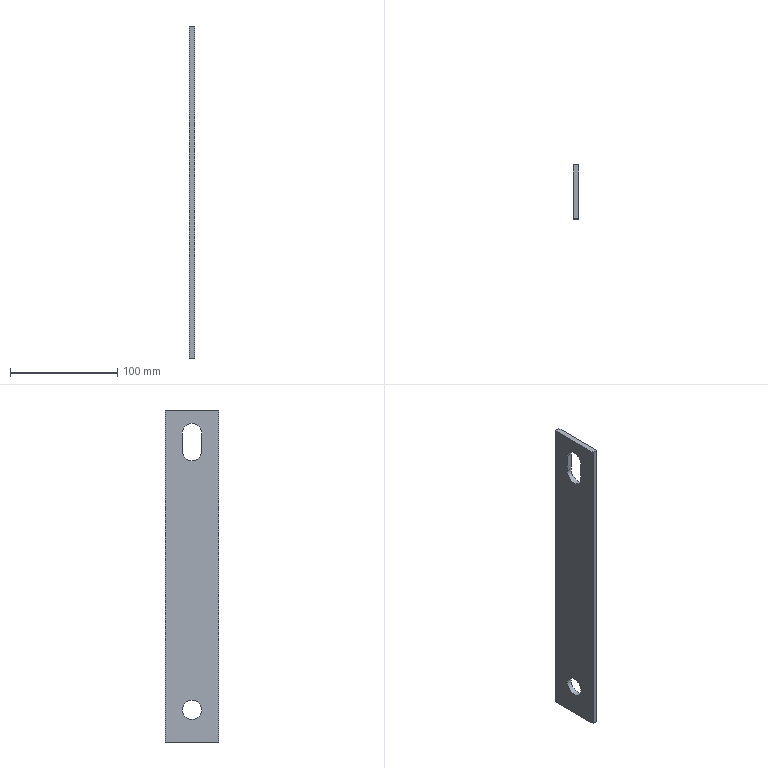Part | NX | features solid 2 | 1 solid | 11 faces | box 5 x 50 x 310 mm | volume 73425 mm3 | plane 8 | cylinder 3 | commonest cylinder face diameters 18 x3
STEP:
#1=CARTESIAN_POINT('',(-1060.,-545.,-129.));
#2=VERTEX_POINT('',#1);
#3=CARTESIAN_POINT('',(-1060.,-545.,181.));
#4=VERTEX_POINT('',#3);
#5=CARTESIAN_POINT('',(-1060.,-545.,-129.));
#6=DIRECTION('',(0.,0.,1.));
#7=VECTOR('',#6,1000.);
#8=LINE('',#5,#7);
#9=EDGE_CURVE('',#2,#4,#8,.T.);
#10=ORIENTED_EDGE('',*,*,#9,.T.);
#11=CARTESIAN_POINT('',(-1065.,-545.,181.));
#12=VERTEX_POINT('',#11);
#13=CARTESIAN_POINT('',(-1065.,-545.,181.));
#14=DIRECTION('',(1.,0.,0.));
#15=VECTOR('',#14,1000.);
#16=LINE('',#13,#15);
#17=EDGE_CURVE('',#12,#4,#16,.T.);
#18=ORIENTED_EDGE('',*,*,#17,.F.);
#19=CARTESIAN_POINT('',(-1065.,-545.,-129.));
#20=VERTEX_POINT('',#19);
#21=CARTESIAN_POINT('',(-1065.,-545.,-129.));
#22=DIRECTION('',(0.,0.,1.));
#23=VECTOR('',#22,1000.);
#24=LINE('',#21,#23);
#25=EDGE_CURVE('',#20,#12,#24,.T.);
#26=ORIENTED_EDGE('',*,*,#25,.F.);
#27=CARTESIAN_POINT('',(-1065.,-545.,-129.));
#28=DIRECTION('',(1.,0.,0.));
#29=VECTOR('',#28,1000.);
#30=LINE('',#27,#29);
#31=EDGE_CURVE('',#20,#2,#30,.T.);
#32=ORIENTED_EDGE('',*,*,#31,.T.);
#33=EDGE_LOOP('',(#10,#18,#26,#32));
#34=FACE_BOUND('',#33,.T.);
#35=CARTESIAN_POINT('',(-1065.,-545.,-129.));
#36=DIRECTION('',(0.,-1.,0.));
#37=DIRECTION('',(0.,0.,1.));
#38=AXIS2_PLACEMENT_3D('',#35,#36,#37);
#39=PLANE('',#38);
#40=ADVANCED_FACE('',(#34),#39,.T.);
#41=CARTESIAN_POINT('',(-1060.,-495.,181.));
#42=VERTEX_POINT('',#41);
#43=CARTESIAN_POINT('',(-1060.,-545.,181.));
#44=DIRECTION('',(0.,1.,0.));
#45=VECTOR('',#44,1000.);
#46=LINE('',#43,#45);
#47=EDGE_CURVE('',#4,#42,#46,.T.);
#48=ORIENTED_EDGE('',*,*,#47,.T.);
#49=CARTESIAN_POINT('',(-1065.,-495.,181.));
#50=VERTEX_POINT('',#49);
#51=CARTESIAN_POINT('',(-1065.,-495.,181.));
#52=DIRECTION('',(1.,0.,0.));
#53=VECTOR('',#52,1000.);
#54=LINE('',#51,#53);
#55=EDGE_CURVE('',#50,#42,#54,.T.);
#56=ORIENTED_EDGE('',*,*,#55,.F.);
#57=CARTESIAN_POINT('',(-1065.,-545.,181.));
#58=DIRECTION('',(0.,1.,0.));
#59=VECTOR('',#58,1000.);
#60=LINE('',#57,#59);
#61=EDGE_CURVE('',#12,#50,#60,.T.);
#62=ORIENTED_EDGE('',*,*,#61,.F.);
#63=ORIENTED_EDGE('',*,*,#17,.T.);
#64=EDGE_LOOP('',(#48,#56,#62,#63));
#65=FACE_BOUND('',#64,.T.);
#66=CARTESIAN_POINT('',(-1065.,-545.,181.));
#67=DIRECTION('',(0.,0.,1.));
#68=DIRECTION('',(1.,0.,0.));
#69=AXIS2_PLACEMENT_3D('',#66,#67,#68);
#70=PLANE('',#69);
#71=ADVANCED_FACE('',(#65),#70,.T.);
#72=CARTESIAN_POINT('',(-1060.,-495.,-129.));
#73=VERTEX_POINT('',#72);
#74=CARTESIAN_POINT('',(-1060.,-495.,181.));
#75=DIRECTION('',(0.,0.,-1.));
#76=VECTOR('',#75,1000.);
#77=LINE('',#74,#76);
#78=EDGE_CURVE('',#42,#73,#77,.T.);
#79=ORIENTED_EDGE('',*,*,#78,.T.);
#80=CARTESIAN_POINT('',(-1065.,-495.,-129.));
#81=VERTEX_POINT('',#80);
#82=CARTESIAN_POINT('',(-1065.,-495.,-129.));
#83=DIRECTION('',(1.,0.,0.));
#84=VECTOR('',#83,1000.);
#85=LINE('',#82,#84);
#86=EDGE_CURVE('',#81,#73,#85,.T.);
#87=ORIENTED_EDGE('',*,*,#86,.F.);
#88=CARTESIAN_POINT('',(-1065.,-495.,181.));
#89=DIRECTION('',(0.,0.,-1.));
#90=VECTOR('',#89,1000.);
#91=LINE('',#88,#90);
#92=EDGE_CURVE('',#50,#81,#91,.T.);
#93=ORIENTED_EDGE('',*,*,#92,.F.);
#94=ORIENTED_EDGE('',*,*,#55,.T.);
#95=EDGE_LOOP('',(#79,#87,#93,#94));
#96=FACE_BOUND('',#95,.T.);
#97=CARTESIAN_POINT('',(-1065.,-495.,181.));
#98=DIRECTION('',(0.,1.,0.));
#99=DIRECTION('',(0.,0.,-1.));
#100=AXIS2_PLACEMENT_3D('',#97,#98,#99);
#101=PLANE('',#100);
#102=ADVANCED_FACE('',(#96),#101,.T.);
#103=CARTESIAN_POINT('',(-1060.,-511.,142.5));
#104=VERTEX_POINT('',#103);
#105=CARTESIAN_POINT('',(-1060.,-529.,142.5));
#106=VERTEX_POINT('',#105);
#107=CARTESIAN_POINT('',(-1060.,-520.,142.5));
#108=DIRECTION('',(-1.,0.,0.));
#109=DIRECTION('',(0.,-1.,0.));
#110=AXIS2_PLACEMENT_3D('',#107,#108,#109);
#111=CIRCLE('',#110,9.);
#112=EDGE_CURVE('',#104,#106,#111,.T.);
#113=ORIENTED_EDGE('',*,*,#112,.F.);
#114=CARTESIAN_POINT('',(-1065.,-511.,142.5));
#115=VERTEX_POINT('',#114);
#116=CARTESIAN_POINT('',(-1065.,-511.,142.5));
#117=DIRECTION('',(1.,0.,0.));
#118=VECTOR('',#117,1000.);
#119=LINE('',#116,#118);
#120=EDGE_CURVE('',#115,#104,#119,.T.);
#121=ORIENTED_EDGE('',*,*,#120,.F.);
#122=CARTESIAN_POINT('',(-1065.,-529.,142.5));
#123=VERTEX_POINT('',#122);
#124=CARTESIAN_POINT('',(-1065.,-520.,142.5));
#125=DIRECTION('',(-1.,0.,0.));
#126=DIRECTION('',(0.,-1.,0.));
#127=AXIS2_PLACEMENT_3D('',#124,#125,#126);
#128=CIRCLE('',#127,9.);
#129=EDGE_CURVE('',#115,#123,#128,.T.);
#130=ORIENTED_EDGE('',*,*,#129,.T.);
#131=CARTESIAN_POINT('',(-1065.,-529.,142.5));
#132=DIRECTION('',(1.,0.,0.));
#133=VECTOR('',#132,1000.);
#134=LINE('',#131,#133);
#135=EDGE_CURVE('',#123,#106,#134,.T.);
#136=ORIENTED_EDGE('',*,*,#135,.T.);
#137=EDGE_LOOP('',(#113,#121,#130,#136));
#138=FACE_BOUND('',#137,.T.);
#139=CARTESIAN_POINT('',(-1065.,-520.,142.5));
#140=DIRECTION('',(1.,0.,0.));
#141=DIRECTION('',(0.,-1.,0.));
#142=AXIS2_PLACEMENT_3D('',#139,#140,#141);
#143=CYLINDRICAL_SURFACE('',#142,9.);
#144=ADVANCED_FACE('',(#138),#143,.F.);
#145=CARTESIAN_POINT('',(-1060.,-511.,159.5));
#146=VERTEX_POINT('',#145);
#147=CARTESIAN_POINT('',(-1060.,-511.,142.5));
#148=DIRECTION('',(0.,0.,1.));
#149=VECTOR('',#148,1000.);
#150=LINE('',#147,#149);
#151=EDGE_CURVE('',#104,#146,#150,.T.);
#152=ORIENTED_EDGE('',*,*,#151,.T.);
#153=CARTESIAN_POINT('',(-1065.,-511.,159.5));
#154=VERTEX_POINT('',#153);
#155=CARTESIAN_POINT('',(-1065.,-511.,159.5));
#156=DIRECTION('',(1.,0.,0.));
#157=VECTOR('',#156,1000.);
#158=LINE('',#155,#157);
#159=EDGE_CURVE('',#154,#146,#158,.T.);
#160=ORIENTED_EDGE('',*,*,#159,.F.);
#161=CARTESIAN_POINT('',(-1065.,-511.,142.5));
#162=DIRECTION('',(0.,0.,1.));
#163=VECTOR('',#162,1000.);
#164=LINE('',#161,#163);
#165=EDGE_CURVE('',#115,#154,#164,.T.);
#166=ORIENTED_EDGE('',*,*,#165,.F.);
#167=ORIENTED_EDGE('',*,*,#120,.T.);
#168=EDGE_LOOP('',(#152,#160,#166,#167));
#169=FACE_BOUND('',#168,.T.);
#170=CARTESIAN_POINT('',(-1065.,-511.,142.5));
#171=DIRECTION('',(0.,-1.,0.));
#172=DIRECTION('',(-1.,0.,0.));
#173=AXIS2_PLACEMENT_3D('',#170,#171,#172);
#174=PLANE('',#173);
#175=ADVANCED_FACE('',(#169),#174,.T.);
#176=CARTESIAN_POINT('',(-1060.,-529.,159.5));
#177=VERTEX_POINT('',#176);
#178=CARTESIAN_POINT('',(-1060.,-520.,159.5));
#179=DIRECTION('',(-1.,0.,0.));
#180=DIRECTION('',(0.,-1.,0.));
#181=AXIS2_PLACEMENT_3D('',#178,#179,#180);
#182=CIRCLE('',#181,9.);
#183=EDGE_CURVE('',#177,#146,#182,.T.);
#184=ORIENTED_EDGE('',*,*,#183,.F.);
#185=CARTESIAN_POINT('',(-1065.,-529.,159.5));
#186=VERTEX_POINT('',#185);
#187=CARTESIAN_POINT('',(-1065.,-529.,159.5));
#188=DIRECTION('',(1.,0.,0.));
#189=VECTOR('',#188,1000.);
#190=LINE('',#187,#189);
#191=EDGE_CURVE('',#186,#177,#190,.T.);
#192=ORIENTED_EDGE('',*,*,#191,.F.);
#193=CARTESIAN_POINT('',(-1065.,-520.,159.5));
#194=DIRECTION('',(-1.,0.,0.));
#195=DIRECTION('',(0.,-1.,0.));
#196=AXIS2_PLACEMENT_3D('',#193,#194,#195);
#197=CIRCLE('',#196,9.);
#198=EDGE_CURVE('',#186,#154,#197,.T.);
#199=ORIENTED_EDGE('',*,*,#198,.T.);
#200=ORIENTED_EDGE('',*,*,#159,.T.);
#201=EDGE_LOOP('',(#184,#192,#199,#200));
#202=FACE_BOUND('',#201,.T.);
#203=CARTESIAN_POINT('',(-1065.,-520.,159.5));
#204=DIRECTION('',(1.,0.,0.));
#205=DIRECTION('',(0.,-1.,0.));
#206=AXIS2_PLACEMENT_3D('',#203,#204,#205);
#207=CYLINDRICAL_SURFACE('',#206,9.);
#208=ADVANCED_FACE('',(#202),#207,.F.);
#209=CARTESIAN_POINT('',(-1060.,-529.,159.5));
#210=DIRECTION('',(0.,0.,-1.));
#211=VECTOR('',#210,1000.);
#212=LINE('',#209,#211);
#213=EDGE_CURVE('',#177,#106,#212,.T.);
#214=ORIENTED_EDGE('',*,*,#213,.T.);
#215=ORIENTED_EDGE('',*,*,#135,.F.);
#216=CARTESIAN_POINT('',(-1065.,-529.,159.5));
#217=DIRECTION('',(0.,0.,-1.));
#218=VECTOR('',#217,1000.);
#219=LINE('',#216,#218);
#220=EDGE_CURVE('',#186,#123,#219,.T.);
#221=ORIENTED_EDGE('',*,*,#220,.F.);
#222=ORIENTED_EDGE('',*,*,#191,.T.);
#223=EDGE_LOOP('',(#214,#215,#221,#222));
#224=FACE_BOUND('',#223,.T.);
#225=CARTESIAN_POINT('',(-1065.,-529.,159.5));
#226=DIRECTION('',(0.,1.,0.));
#227=DIRECTION('',(1.,0.,0.));
#228=AXIS2_PLACEMENT_3D('',#225,#226,#227);
#229=PLANE('',#228);
#230=ADVANCED_FACE('',(#224),#229,.T.);
#231=CARTESIAN_POINT('',(-1065.,-529.,-99.));
#232=VERTEX_POINT('',#231);
#233=CARTESIAN_POINT('',(-1065.,-520.,-99.));
#234=DIRECTION('',(-1.,0.,0.));
#235=DIRECTION('',(0.,-1.,0.));
#236=AXIS2_PLACEMENT_3D('',#233,#234,#235);
#237=CIRCLE('',#236,9.);
#238=EDGE_CURVE('',#232,#232,#237,.T.);
#239=ORIENTED_EDGE('',*,*,#238,.T.);
#240=EDGE_LOOP('',(#239));
#241=FACE_BOUND('',#240,.T.);
#242=CARTESIAN_POINT('',(-1060.,-529.,-99.));
#243=VERTEX_POINT('',#242);
#244=CARTESIAN_POINT('',(-1060.,-520.,-99.));
#245=DIRECTION('',(-1.,0.,0.));
#246=DIRECTION('',(0.,-1.,0.));
#247=AXIS2_PLACEMENT_3D('',#244,#245,#246);
#248=CIRCLE('',#247,9.);
#249=EDGE_CURVE('',#243,#243,#248,.T.);
#250=ORIENTED_EDGE('',*,*,#249,.F.);
#251=EDGE_LOOP('',(#250));
#252=FACE_BOUND('',#251,.T.);
#253=CARTESIAN_POINT('',(-1065.,-520.,-99.));
#254=DIRECTION('',(1.,0.,0.));
#255=DIRECTION('',(0.,-1.,0.));
#256=AXIS2_PLACEMENT_3D('',#253,#254,#255);
#257=CYLINDRICAL_SURFACE('',#256,9.);
#258=ADVANCED_FACE('',(#241,#252),#257,.F.);
#259=CARTESIAN_POINT('',(-1060.,-495.,-129.));
#260=DIRECTION('',(0.,-1.,0.));
#261=VECTOR('',#260,1000.);
#262=LINE('',#259,#261);
#263=EDGE_CURVE('',#73,#2,#262,.T.);
#264=ORIENTED_EDGE('',*,*,#263,.T.);
#265=ORIENTED_EDGE('',*,*,#31,.F.);
#266=CARTESIAN_POINT('',(-1065.,-495.,-129.));
#267=DIRECTION('',(0.,-1.,0.));
#268=VECTOR('',#267,1000.);
#269=LINE('',#266,#268);
#270=EDGE_CURVE('',#81,#20,#269,.T.);
#271=ORIENTED_EDGE('',*,*,#270,.F.);
#272=ORIENTED_EDGE('',*,*,#86,.T.);
#273=EDGE_LOOP('',(#264,#265,#271,#272));
#274=FACE_BOUND('',#273,.T.);
#275=CARTESIAN_POINT('',(-1065.,-495.,-129.));
#276=DIRECTION('',(0.,0.,-1.));
#277=DIRECTION('',(-1.,0.,0.));
#278=AXIS2_PLACEMENT_3D('',#275,#276,#277);
#279=PLANE('',#278);
#280=ADVANCED_FACE('',(#274),#279,.T.);
#281=ORIENTED_EDGE('',*,*,#238,.F.);
#282=EDGE_LOOP('',(#281));
#283=FACE_BOUND('',#282,.T.);
#284=ORIENTED_EDGE('',*,*,#129,.F.);
#285=ORIENTED_EDGE('',*,*,#165,.T.);
#286=ORIENTED_EDGE('',*,*,#198,.F.);
#287=ORIENTED_EDGE('',*,*,#220,.T.);
#288=EDGE_LOOP('',(#284,#285,#286,#287));
#289=FACE_BOUND('',#288,.T.);
#290=ORIENTED_EDGE('',*,*,#25,.T.);
#291=ORIENTED_EDGE('',*,*,#61,.T.);
#292=ORIENTED_EDGE('',*,*,#92,.T.);
#293=ORIENTED_EDGE('',*,*,#270,.T.);
#294=EDGE_LOOP('',(#290,#291,#292,#293));
#295=FACE_BOUND('',#294,.T.);
#296=CARTESIAN_POINT('',(-1065.,-545.,181.));
#297=DIRECTION('',(1.,0.,0.));
#298=DIRECTION('',(0.,-1.,0.));
#299=AXIS2_PLACEMENT_3D('',#296,#297,#298);
#300=PLANE('',#299);
#301=ADVANCED_FACE('',(#283,#289,#295),#300,.F.);
#302=ORIENTED_EDGE('',*,*,#249,.T.);
#303=EDGE_LOOP('',(#302));
#304=FACE_BOUND('',#303,.T.);
#305=ORIENTED_EDGE('',*,*,#112,.T.);
#306=ORIENTED_EDGE('',*,*,#213,.F.);
#307=ORIENTED_EDGE('',*,*,#183,.T.);
#308=ORIENTED_EDGE('',*,*,#151,.F.);
#309=EDGE_LOOP('',(#305,#306,#307,#308));
#310=FACE_BOUND('',#309,.T.);
#311=ORIENTED_EDGE('',*,*,#9,.F.);
#312=ORIENTED_EDGE('',*,*,#263,.F.);
#313=ORIENTED_EDGE('',*,*,#78,.F.);
#314=ORIENTED_EDGE('',*,*,#47,.F.);
#315=EDGE_LOOP('',(#311,#312,#313,#314));
#316=FACE_BOUND('',#315,.T.);
#317=CARTESIAN_POINT('',(-1060.,-545.,181.));
#318=DIRECTION('',(1.,0.,0.));
#319=DIRECTION('',(0.,-1.,0.));
#320=AXIS2_PLACEMENT_3D('',#317,#318,#319);
#321=PLANE('',#320);
#322=ADVANCED_FACE('',(#304,#310,#316),#321,.T.);
#323=CLOSED_SHELL('',(#40,#71,#102,#144,#175,#208,#230,#258,#280,#301,#322));
#324=MANIFOLD_SOLID_BREP('',#323);
#325=(LENGTH_UNIT()NAMED_UNIT(*)SI_UNIT(.MILLI.,.METRE.));
#326=UNCERTAINTY_MEASURE_WITH_UNIT(LENGTH_MEASURE(0.00001),#325,'','');
#327=(NAMED_UNIT(*)PLANE_ANGLE_UNIT()SI_UNIT($,.RADIAN.));
#328=(NAMED_UNIT(*)SI_UNIT($,.STERADIAN.)SOLID_ANGLE_UNIT());
#329=(GEOMETRIC_REPRESENTATION_CONTEXT(3)GLOBAL_UNCERTAINTY_ASSIGNED_CONTEXT((#326))GLOBAL_UNIT_ASSIGNED_CONTEXT((#325,#327,#328))REPRESENTATION_CONTEXT('',''));
#330=ADVANCED_BREP_SHAPE_REPRESENTATION('',(#324),#329);